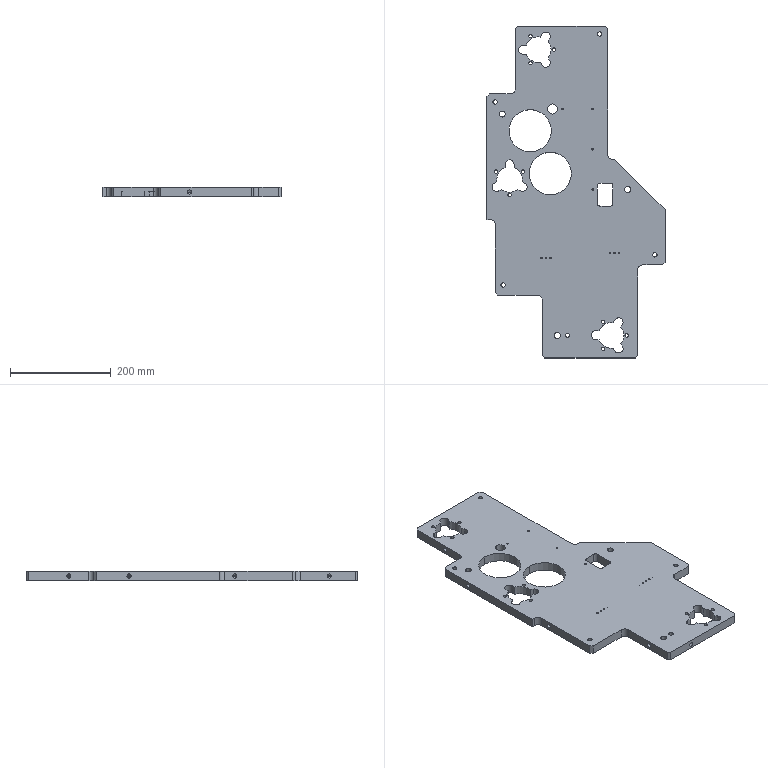NC program | NX | posted with a generic post | part box 354 x 660 x 18 mm
Lines 1 to 41 of 43361:
N10 G17 G21 G94 G90
(DRILLING , TOOL : ZXZ)
N12 T01 M6
N14 G54
N16 G17 G0 G90 X283. Y-44. S3000 M3
N18 G43 Z30. H1
N20 G94 G81 G98 Z-1. F250. R3.
N22 X309.847 Y-90.5
N24 X256.153
N26 X40.5 Y-105.153
N28 Y-158.847
N30 X-6. Y-132.
N32 X-258.153 Y54.11
N34 X-285. Y100.61
N36 X-311.847 Y54.11
N38 G80
N40 G0 X-311.847 Y54.11 Z30.
N42 M5
(DRILLING_COPY , TOOL : 6.8ZT)
N44 T06 M6
N46 G54
N48 G17 G0 G90 X283. Y-44. S2000 M3
N50 G43 Z30. H6
N52 G94 G83 G98 Z-21.543 F150. Q2. R3.
N54 X309.847 Y-90.5
N56 X256.153
N58 X40.5 Y-105.153
N60 Y-158.847
N62 X-6. Y-132.
N64 X-258.153 Y54.11
N66 X-285. Y100.61
N68 X-311.847 Y54.11
N70 G80
N72 G0 X-311.847 Y54.11 Z30.
N74 M5